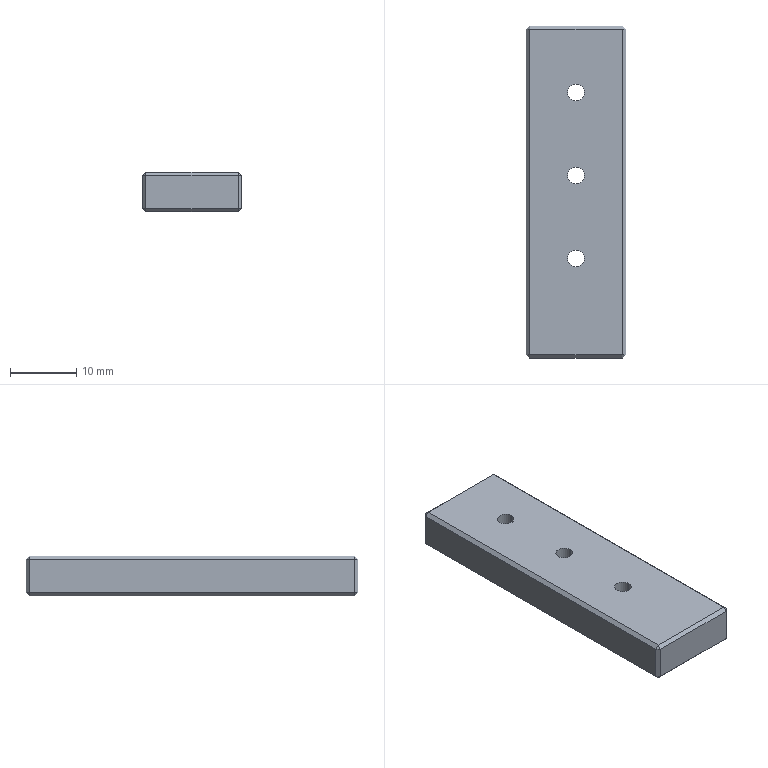Part | STEP file | BPSP-11-21 Bumper Block_Default | 1 solid | 32 faces | box 15 x 50 x 6 mm | volume 4377 mm3 | plane 26 | cylinder 6 | commonest cylinder face diameters 2.5 x6